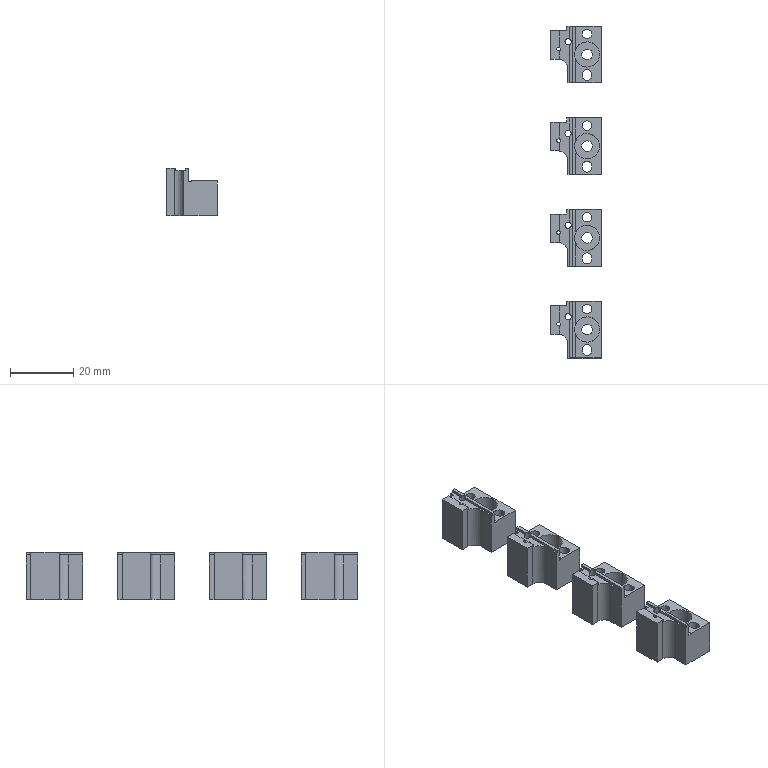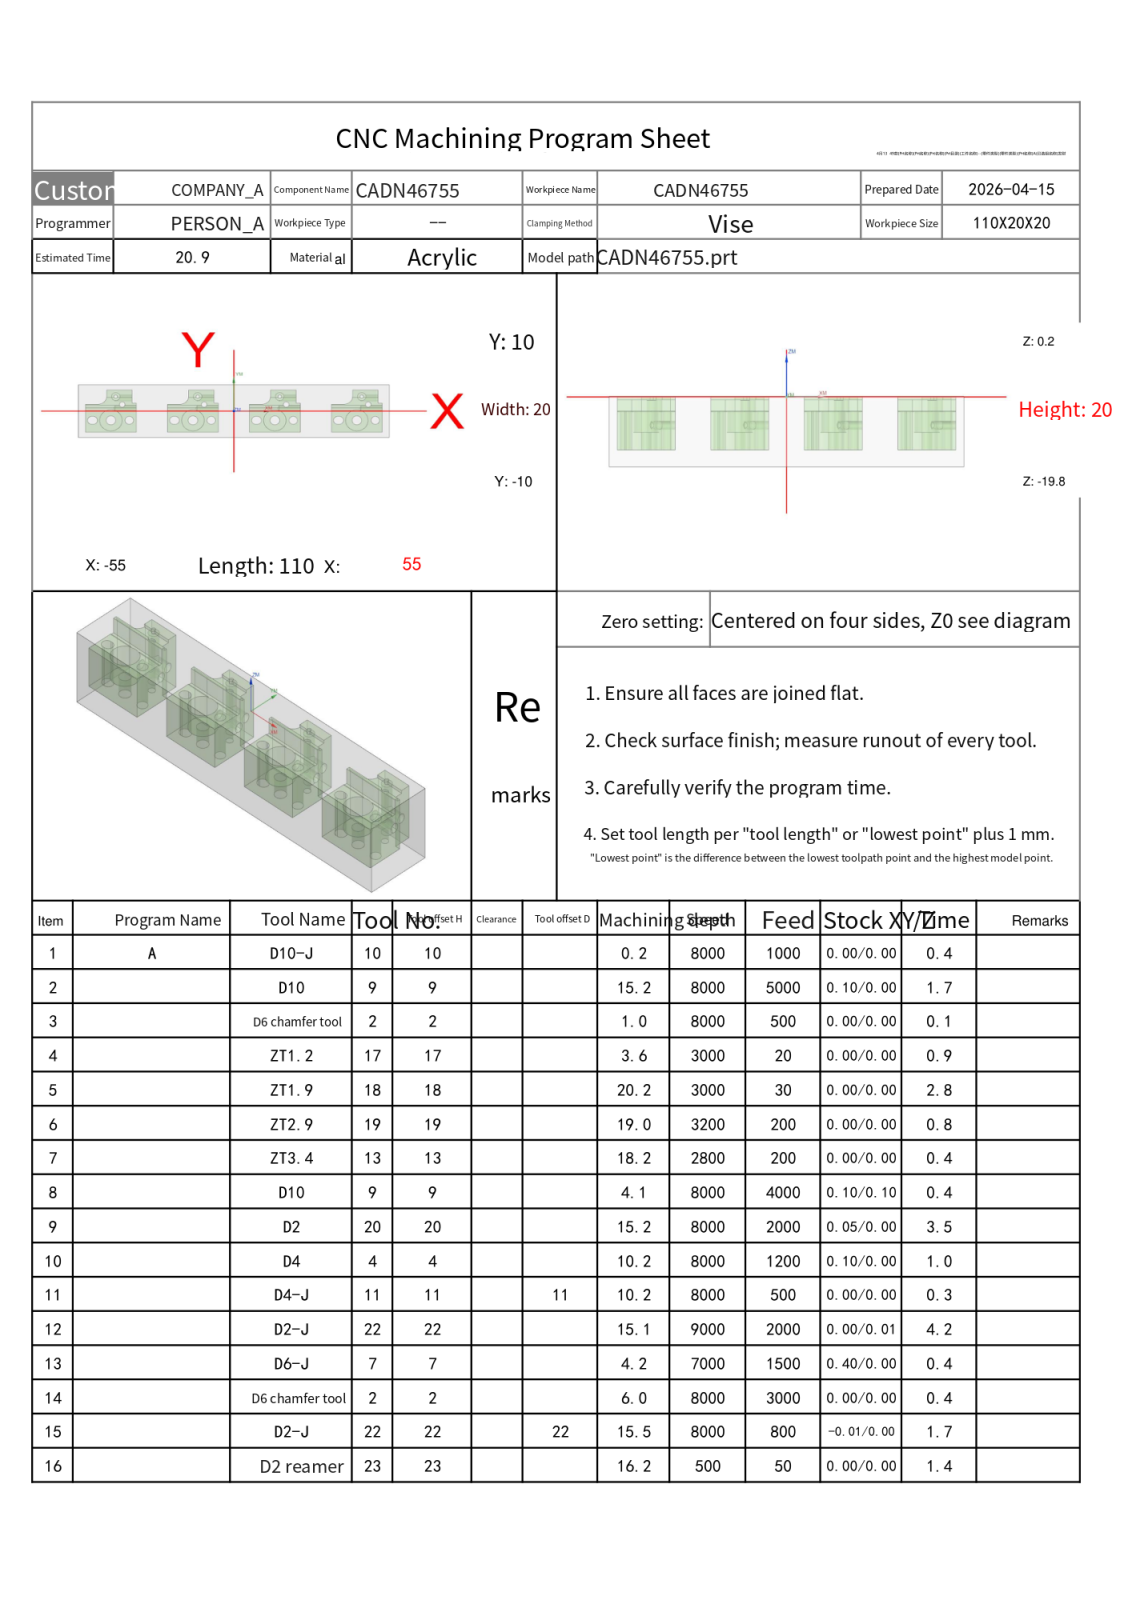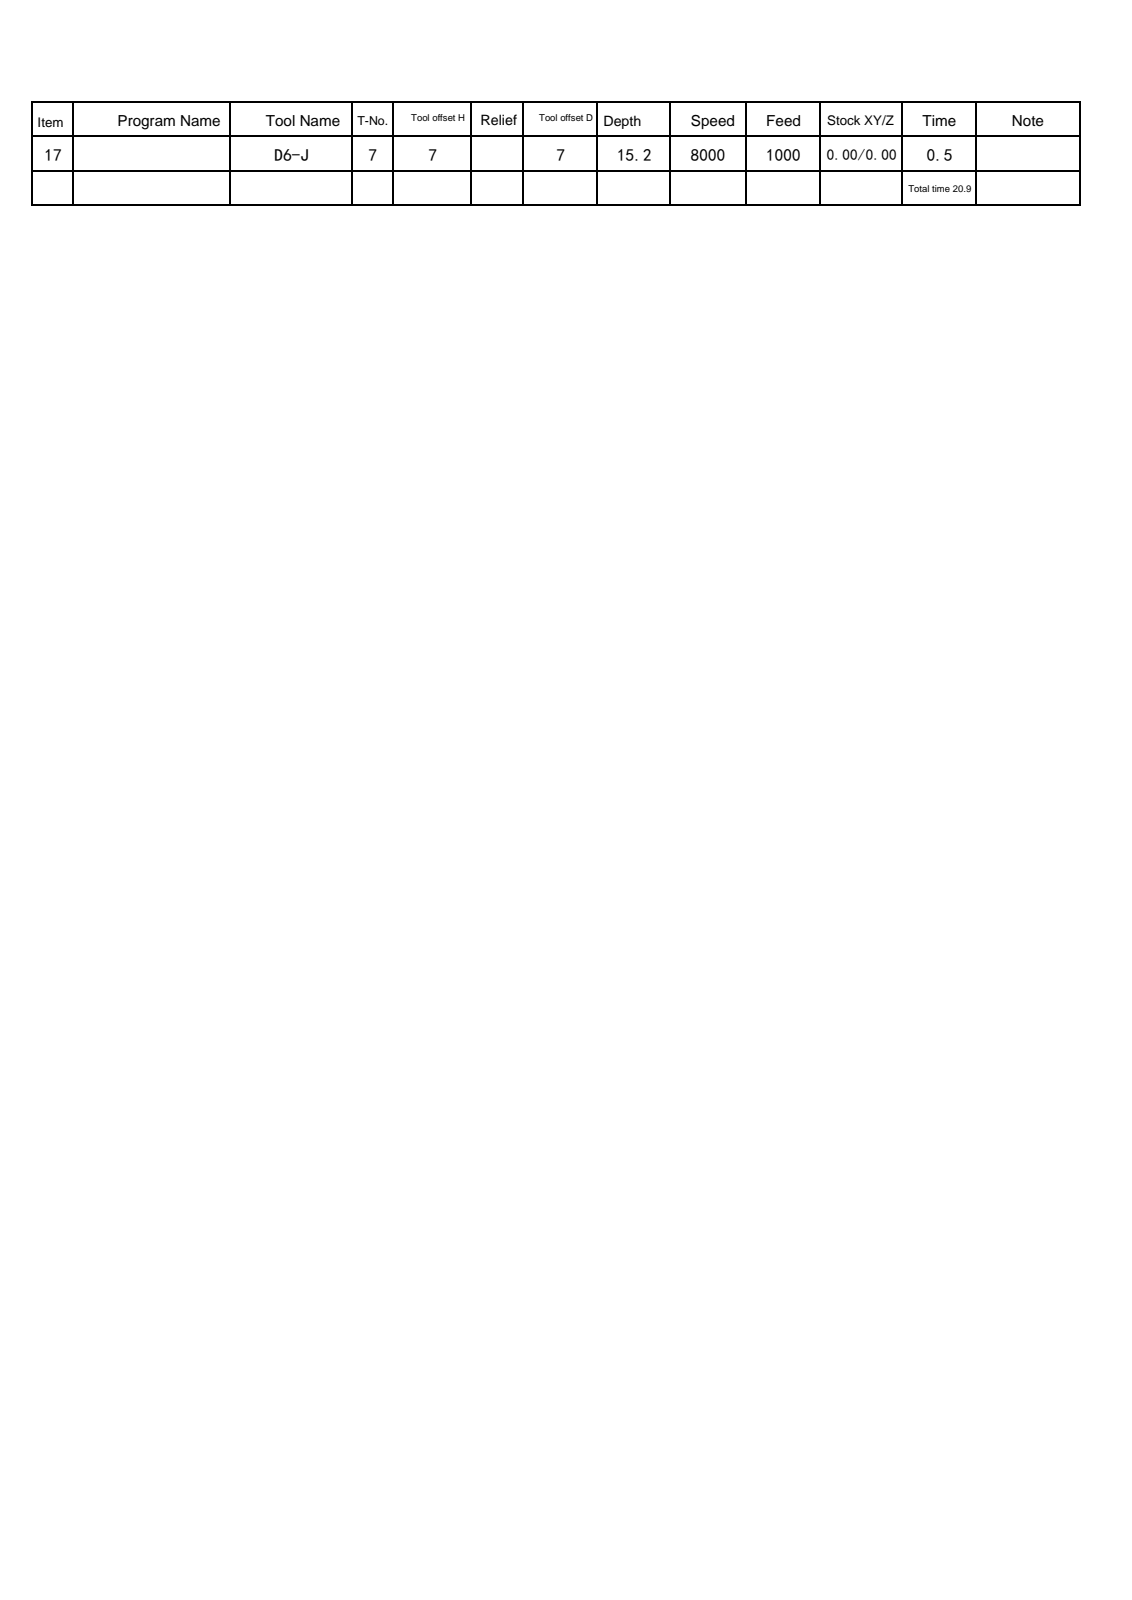NC program | NX | posted by the shop | part box 16 x 105 x 15 mm
Lines 5249 to 5478 of 25120:
N10 T04 M06
(D4  D=4. R=0. H=04 ce=0.10 di=0.00)
G00 G90 G54 X14.5 Y-3.5 M03 S8000
G43 H04 Z20.
M08
Z-3.5
G03 X13.55 Y-4.45 I0.0 J-.95 F1200.
X14.5 Y-5.4 I.95 J0.0
X14.5 Y-5.4 Z-3.8 I0.0 J1.9
X14.5 Y-5.4 Z-4.1 I0.0 J1.9
X14.5 Y-5.4 Z-4.4 I0.0 J1.9
X14.5 Y-5.4 Z-4.7 I0.0 J1.9
X14.5 Y-5.4 Z-5. I0.0 J1.9
X14.5 Y-5.4 Z-5.3 I0.0 J1.9
X14.5 Y-5.4 Z-5.6 I0.0 J1.9
X14.5 Y-5.4 Z-5.9 I0.0 J1.9
X14.5 Y-5.4 Z-6.2 I0.0 J1.9
X14.5 Y-5.4 Z-6.5 I0.0 J1.9
X14.5 Y-5.4 Z-6.8 I0.0 J1.9
X14.5 Y-5.4 Z-7.1 I0.0 J1.9
X14.5 Y-5.4 Z-7.4 I0.0 J1.9
X14.5 Y-5.4 Z-7.7 I0.0 J1.9
X14.5 Y-5.4 Z-8. I0.0 J1.9
X14.5 Y-5.4 Z-8.3 I0.0 J1.9
X14.5 Y-5.4 Z-8.6 I0.0 J1.9
X14.5 Y-5.4 Z-8.9 I0.0 J1.9
X14.5 Y-5.4 Z-9.2 I0.0 J1.9
X14.5 Y-5.4 Z-9.5 I0.0 J1.9
X14.5 Y-5.4 Z-9.8 I0.0 J1.9
X12.855 Y-2.55 Z-10. I0.0 J1.9
X12.6 Y-3.5 I1.645 J-.95
X14.5 Y-5.4 I1.9 J0.0
X16.4 Y-3.5 I0.0 J1.9
X14.5 Y-1.6 I-1.9 J0.0
X12.855 Y-2.55 I0.0 J-1.9
X12.727 Y-3.025 I.823 J-.475
X13.677 Y-3.975 I.95 J0.0
X14.5 Y-3.5 I0.0 J.95
G00 Z20.
X43.5
Z-3.5
G03 X42.55 Y-4.45 I0.0 J-.95
X43.5 Y-5.4 I.95 J0.0
X43.5 Y-5.4 Z-3.8 I0.0 J1.9
X43.5 Y-5.4 Z-4.1 I0.0 J1.9
X43.5 Y-5.4 Z-4.4 I0.0 J1.9
X43.5 Y-5.4 Z-4.7 I0.0 J1.9
X43.5 Y-5.4 Z-5. I0.0 J1.9
X43.5 Y-5.4 Z-5.3 I0.0 J1.9
X43.5 Y-5.4 Z-5.6 I0.0 J1.9
X43.5 Y-5.4 Z-5.9 I0.0 J1.9
X43.5 Y-5.4 Z-6.2 I0.0 J1.9
X43.5 Y-5.4 Z-6.5 I0.0 J1.9
X43.5 Y-5.4 Z-6.8 I0.0 J1.9
X43.5 Y-5.4 Z-7.1 I0.0 J1.9
X43.5 Y-5.4 Z-7.4 I0.0 J1.9
X43.5 Y-5.4 Z-7.7 I0.0 J1.9
X43.5 Y-5.4 Z-8. I0.0 J1.9
X43.5 Y-5.4 Z-8.3 I0.0 J1.9
X43.5 Y-5.4 Z-8.6 I0.0 J1.9
X43.5 Y-5.4 Z-8.9 I0.0 J1.9
X43.5 Y-5.4 Z-9.2 I0.0 J1.9
X43.5 Y-5.4 Z-9.5 I0.0 J1.9
X43.5 Y-5.4 Z-9.8 I0.0 J1.9
X41.855 Y-2.55 Z-10. I0.0 J1.9
X41.6 Y-3.5 I1.645 J-.95
X43.5 Y-5.4 I1.9 J0.0
X45.4 Y-3.5 I0.0 J1.9
X43.5 Y-1.6 I-1.9 J0.0
X41.855 Y-2.55 I0.0 J-1.9
X41.727 Y-3.025 I.823 J-.475
X42.677 Y-3.975 I.95 J0.0
X43.5 Y-3.5 I0.0 J.95
G00 Z20.
X-14.5
Z-3.5
G03 X-15.45 Y-4.45 I0.0 J-.95
X-14.5 Y-5.4 I.95 J0.0
X-14.5 Y-5.4 Z-3.8 I0.0 J1.9
X-14.5 Y-5.4 Z-4.1 I0.0 J1.9
X-14.5 Y-5.4 Z-4.4 I0.0 J1.9
X-14.5 Y-5.4 Z-4.7 I0.0 J1.9
X-14.5 Y-5.4 Z-5. I0.0 J1.9
X-14.5 Y-5.4 Z-5.3 I0.0 J1.9
X-14.5 Y-5.4 Z-5.6 I0.0 J1.9
X-14.5 Y-5.4 Z-5.9 I0.0 J1.9
X-14.5 Y-5.4 Z-6.2 I0.0 J1.9
X-14.5 Y-5.4 Z-6.5 I0.0 J1.9
X-14.5 Y-5.4 Z-6.8 I0.0 J1.9
X-14.5 Y-5.4 Z-7.1 I0.0 J1.9
X-14.5 Y-5.4 Z-7.4 I0.0 J1.9
X-14.5 Y-5.4 Z-7.7 I0.0 J1.9
X-14.5 Y-5.4 Z-8. I0.0 J1.9
X-14.5 Y-5.4 Z-8.3 I0.0 J1.9
X-14.5 Y-5.4 Z-8.6 I0.0 J1.9
X-14.5 Y-5.4 Z-8.9 I0.0 J1.9
X-14.5 Y-5.4 Z-9.2 I0.0 J1.9
X-14.5 Y-5.4 Z-9.5 I0.0 J1.9
X-14.5 Y-5.4 Z-9.8 I0.0 J1.9
X-16.145 Y-2.55 Z-10. I0.0 J1.9
X-16.4 Y-3.5 I1.645 J-.95
X-14.5 Y-5.4 I1.9 J0.0
X-12.6 Y-3.5 I0.0 J1.9
X-14.5 Y-1.6 I-1.9 J0.0
X-16.145 Y-2.55 I0.0 J-1.9
X-16.273 Y-3.025 I.823 J-.475
X-15.323 Y-3.975 I.95 J0.0
X-14.5 Y-3.5 I0.0 J.95
G00 Z20.
X-43.5
Z-3.5
G03 X-44.45 Y-4.45 I0.0 J-.95
X-43.5 Y-5.4 I.95 J0.0
X-43.5 Y-5.4 Z-3.8 I0.0 J1.9
X-43.5 Y-5.4 Z-4.1 I0.0 J1.9
X-43.5 Y-5.4 Z-4.4 I0.0 J1.9
X-43.5 Y-5.4 Z-4.7 I0.0 J1.9
X-43.5 Y-5.4 Z-5. I0.0 J1.9
X-43.5 Y-5.4 Z-5.3 I0.0 J1.9
X-43.5 Y-5.4 Z-5.6 I0.0 J1.9
X-43.5 Y-5.4 Z-5.9 I0.0 J1.9
X-43.5 Y-5.4 Z-6.2 I0.0 J1.9
X-43.5 Y-5.4 Z-6.5 I0.0 J1.9
X-43.5 Y-5.4 Z-6.8 I0.0 J1.9
X-43.5 Y-5.4 Z-7.1 I0.0 J1.9
X-43.5 Y-5.4 Z-7.4 I0.0 J1.9
X-43.5 Y-5.4 Z-7.7 I0.0 J1.9
X-43.5 Y-5.4 Z-8. I0.0 J1.9
X-43.5 Y-5.4 Z-8.3 I0.0 J1.9
X-43.5 Y-5.4 Z-8.6 I0.0 J1.9
X-43.5 Y-5.4 Z-8.9 I0.0 J1.9
X-43.5 Y-5.4 Z-9.2 I0.0 J1.9
X-43.5 Y-5.4 Z-9.5 I0.0 J1.9
X-43.5 Y-5.4 Z-9.8 I0.0 J1.9
X-45.145 Y-2.55 Z-10. I0.0 J1.9
X-45.4 Y-3.5 I1.645 J-.95
X-43.5 Y-5.4 I1.9 J0.0
X-41.6 Y-3.5 I0.0 J1.9
X-43.5 Y-1.6 I-1.9 J0.0
X-45.145 Y-2.55 I0.0 J-1.9
X-45.273 Y-3.025 I.823 J-.475
X-44.323 Y-3.975 I.95 J0.0
X-43.5 Y-3.5 I0.0 J.95
G00 Z20.
G91 G28 Z0.0
M05
M09
G91 G28 Z0.0
M01
N11 T11 M06
(D4-J  D=4. R=0. H=11 ce=0.00 di=0.00)
G00 G90 G54 X14.5 Y-3.5 M03 S8000
G43 H11 Z20.
M08
Z-3.5
G41 D11
G01 X14.304 Y-3.54 F500.
G03 X13.51 Y-4.51 I.196 J-.97
X14.5 Y-5.5 I.99 J0.0
X14.5 Y-5.5 Z-8.5 I0.0 J2.
X16.402 Y-2.882 Z-10. I0.0 J2.
X14.5 Y-1.5 I-1.902 J-.618
X12.5 Y-3.5 I0.0 J-2.
X14.5 Y-5.5 I2. J0.0
X16.5 Y-3.5 I0.0 J2.
X16.402 Y-2.882 I-2. J0.0
X15.461 Y-2.198 I-.942 J-.306
X14.471 Y-3.188 I0.0 J-.99
G01 X14.477 Y-3.301
G40 X14.5 Y-3.5
G00 Z20.
X43.5
Z-3.5
G41 D11
G01 X43.304 Y-3.54
G03 X42.51 Y-4.51 I.196 J-.97
X43.5 Y-5.5 I.99 J0.0
X43.5 Y-5.5 Z-8.5 I0.0 J2.
X45.402 Y-2.882 Z-10. I0.0 J2.
X43.5 Y-1.5 I-1.902 J-.618
X41.5 Y-3.5 I0.0 J-2.
X43.5 Y-5.5 I2. J0.0
X45.5 Y-3.5 I0.0 J2.
X45.402 Y-2.882 I-2. J0.0
X44.461 Y-2.198 I-.942 J-.306
X43.471 Y-3.188 I0.0 J-.99
G01 X43.477 Y-3.301
G40 X43.5 Y-3.5
G00 Z20.
X-14.5
Z-3.5
G41 D11
G01 X-14.696 Y-3.54
G03 X-15.49 Y-4.51 I.196 J-.97
X-14.5 Y-5.5 I.99 J0.0
X-14.5 Y-5.5 Z-8.5 I0.0 J2.
X-12.598 Y-2.882 Z-10. I0.0 J2.
X-14.5 Y-1.5 I-1.902 J-.618
X-16.5 Y-3.5 I0.0 J-2.
X-14.5 Y-5.5 I2. J0.0
X-12.5 Y-3.5 I0.0 J2.
X-12.598 Y-2.882 I-2. J0.0
X-13.539 Y-2.198 I-.942 J-.306
X-14.529 Y-3.188 I0.0 J-.99
G01 X-14.523 Y-3.301
G40 X-14.5 Y-3.5
G00 Z20.
X-43.5
Z-3.5
G41 D11
G01 X-43.696 Y-3.54
G03 X-44.49 Y-4.51 I.196 J-.97
X-43.5 Y-5.5 I.99 J0.0
X-43.5 Y-5.5 Z-8.5 I0.0 J2.
X-41.598 Y-2.882 Z-10. I0.0 J2.
X-43.5 Y-1.5 I-1.902 J-.618
X-45.5 Y-3.5 I0.0 J-2.
X-43.5 Y-5.5 I2. J0.0
X-41.5 Y-3.5 I0.0 J2.
X-41.598 Y-2.882 I-2. J0.0
X-42.539 Y-2.198 I-.942 J-.306
X-43.529 Y-3.188 I0.0 J-.99
G01 X-43.523 Y-3.301
G40 X-43.5 Y-3.5
G00 Z20.
G91 G28 Z0.0
M05
M09
G91 G28 Z0.0
M01